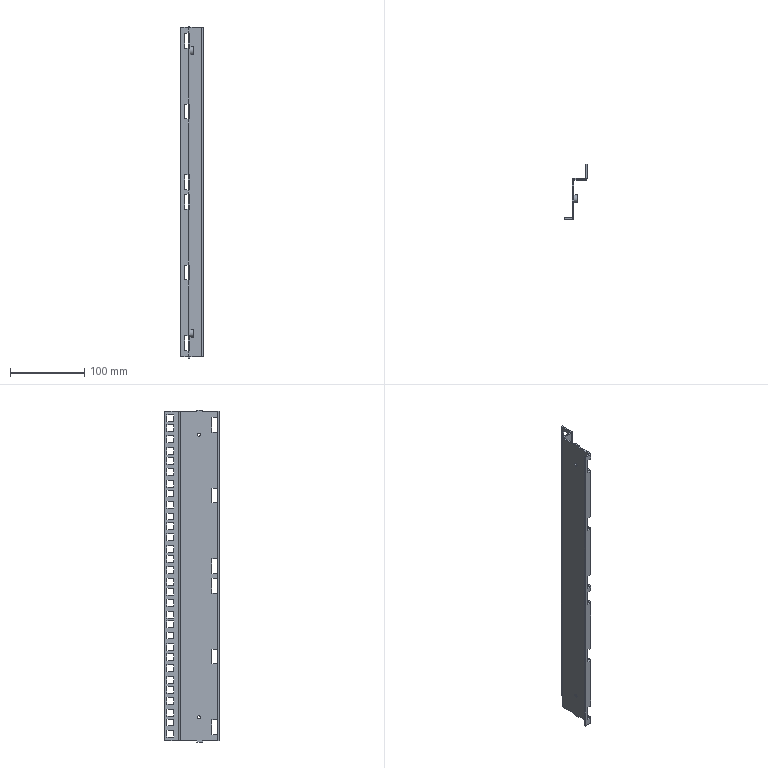Part | STEP file | FHD-021-001-N rack welded part N | 1 solid | 188 faces | box 30 x 73.5 x 446.5 mm | volume 80480 mm3 | plane 166 | cylinder 22 | commonest cylinder face diameters 0.4 x9 4.4 x9 4.2 x2 10.2 x2